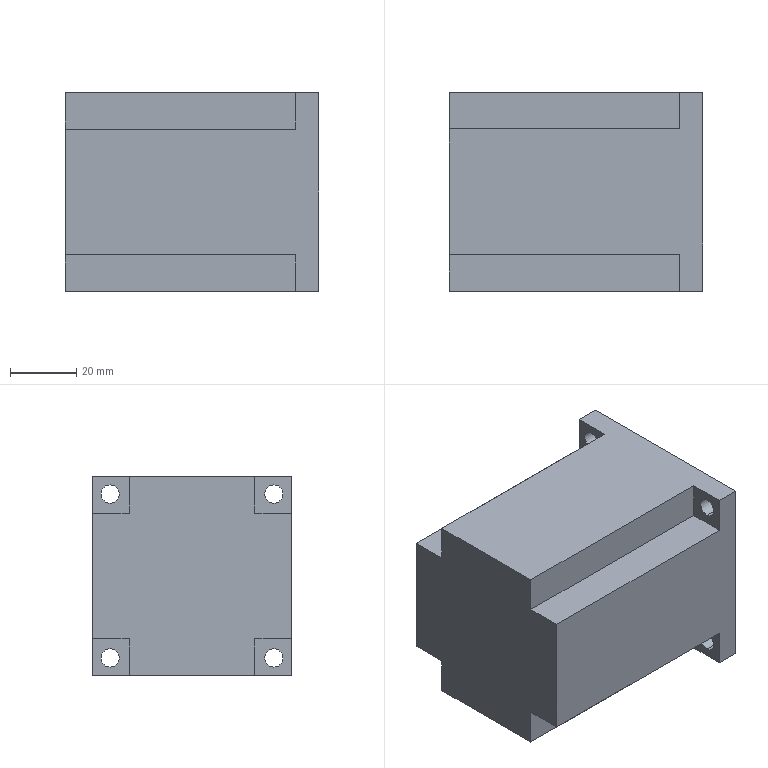Part | STEP file | 0245_Z_101_HF-MP23_1 | 1 solid | 26 faces | box 76.6 x 60 x 60 mm | volume 241408 mm3 | plane 18 | cylinder 8 | commonest cylinder face diameters 5.5 x8